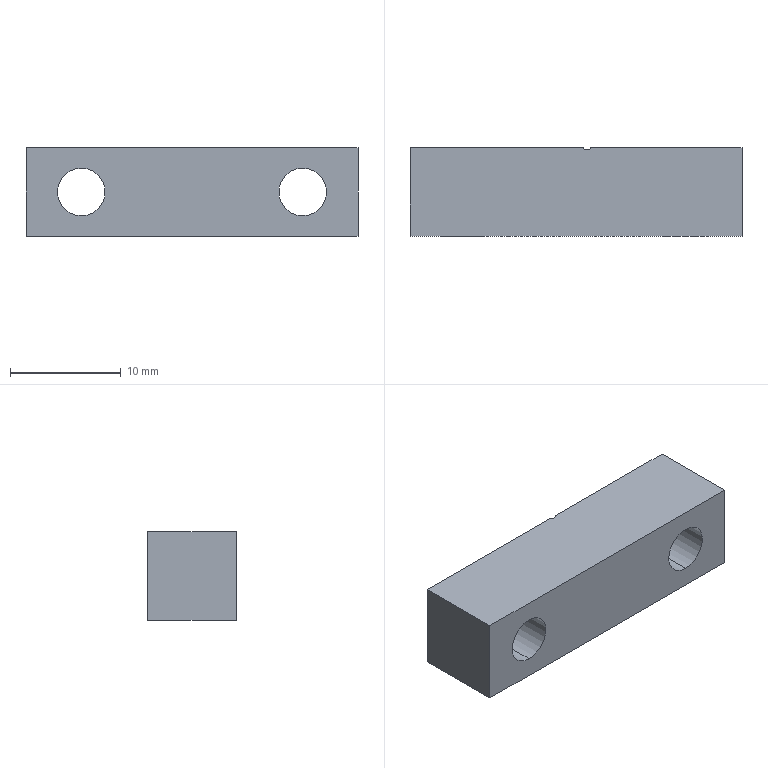Part | SolidWorks | features ICE 2, Extrusion 1 | 1 solid | 12 faces | box 30 x 8 x 8 mm | volume 1687 mm3 | plane 7 | cylinder 5 | commonest cylinder face diameters 4.3 x4 0.8 x1
STEP:
#1=CARTESIAN_POINT('',(-7.907,-5.249,1.85));
#2=VERTEX_POINT('',#1);
#3=CARTESIAN_POINT('',(-7.907,-5.249,6.15));
#4=VERTEX_POINT('',#3);
#5=CARTESIAN_POINT('',(-7.907,-5.249,4.));
#6=DIRECTION('',(0.,1.,0.));
#7=DIRECTION('',(0.,0.,1.));
#8=AXIS2_PLACEMENT_3D('',#5,#6,#7);
#9=CIRCLE('',#8,2.15);
#10=EDGE_CURVE('',#2,#4,#9,.T.);
#11=ORIENTED_EDGE('',*,*,#10,.F.);
#12=CARTESIAN_POINT('',(-7.907,2.751,1.85));
#13=VERTEX_POINT('',#12);
#14=CARTESIAN_POINT('',(-7.907,-5.249,1.85));
#15=DIRECTION('',(0.,1.,0.));
#16=VECTOR('',#15,1000.);
#17=LINE('',#14,#16);
#18=EDGE_CURVE('',#2,#13,#17,.T.);
#19=ORIENTED_EDGE('',*,*,#18,.T.);
#20=CARTESIAN_POINT('',(-7.907,2.751,6.15));
#21=VERTEX_POINT('',#20);
#22=CARTESIAN_POINT('',(-7.907,2.751,4.));
#23=DIRECTION('',(0.,1.,0.));
#24=DIRECTION('',(0.,0.,1.));
#25=AXIS2_PLACEMENT_3D('',#22,#23,#24);
#26=CIRCLE('',#25,2.15);
#27=EDGE_CURVE('',#13,#21,#26,.T.);
#28=ORIENTED_EDGE('',*,*,#27,.T.);
#29=CARTESIAN_POINT('',(-7.907,-5.249,6.15));
#30=DIRECTION('',(0.,1.,0.));
#31=VECTOR('',#30,1000.);
#32=LINE('',#29,#31);
#33=EDGE_CURVE('',#4,#21,#32,.T.);
#34=ORIENTED_EDGE('',*,*,#33,.F.);
#35=EDGE_LOOP('',(#11,#19,#28,#34));
#36=FACE_OUTER_BOUND('',#35,.T.);
#37=CARTESIAN_POINT('',(-7.907,-5.249,4.));
#38=DIRECTION('',(0.,1.,0.));
#39=DIRECTION('',(0.,0.,1.));
#40=AXIS2_PLACEMENT_3D('',#37,#38,#39);
#41=CYLINDRICAL_SURFACE('',#40,2.15);
#42=ADVANCED_FACE('',(#36),#41,.F.);
#43=CARTESIAN_POINT('',(12.093,-5.249,1.85));
#44=VERTEX_POINT('',#43);
#45=CARTESIAN_POINT('',(12.093,-5.249,6.15));
#46=VERTEX_POINT('',#45);
#47=CARTESIAN_POINT('',(12.093,-5.249,4.));
#48=DIRECTION('',(0.,1.,0.));
#49=DIRECTION('',(0.,0.,1.));
#50=AXIS2_PLACEMENT_3D('',#47,#48,#49);
#51=CIRCLE('',#50,2.15);
#52=EDGE_CURVE('',#44,#46,#51,.T.);
#53=ORIENTED_EDGE('',*,*,#52,.F.);
#54=CARTESIAN_POINT('',(12.093,2.751,1.85));
#55=VERTEX_POINT('',#54);
#56=CARTESIAN_POINT('',(12.093,-5.249,1.85));
#57=DIRECTION('',(0.,1.,0.));
#58=VECTOR('',#57,1000.);
#59=LINE('',#56,#58);
#60=EDGE_CURVE('',#44,#55,#59,.T.);
#61=ORIENTED_EDGE('',*,*,#60,.T.);
#62=CARTESIAN_POINT('',(12.093,2.751,6.15));
#63=VERTEX_POINT('',#62);
#64=CARTESIAN_POINT('',(12.093,2.751,4.));
#65=DIRECTION('',(0.,1.,0.));
#66=DIRECTION('',(0.,0.,1.));
#67=AXIS2_PLACEMENT_3D('',#64,#65,#66);
#68=CIRCLE('',#67,2.15);
#69=EDGE_CURVE('',#55,#63,#68,.T.);
#70=ORIENTED_EDGE('',*,*,#69,.T.);
#71=CARTESIAN_POINT('',(12.093,-5.249,6.15));
#72=DIRECTION('',(0.,1.,0.));
#73=VECTOR('',#72,1000.);
#74=LINE('',#71,#73);
#75=EDGE_CURVE('',#46,#63,#74,.T.);
#76=ORIENTED_EDGE('',*,*,#75,.F.);
#77=EDGE_LOOP('',(#53,#61,#70,#76));
#78=FACE_OUTER_BOUND('',#77,.T.);
#79=CARTESIAN_POINT('',(12.093,-5.249,4.));
#80=DIRECTION('',(0.,1.,0.));
#81=DIRECTION('',(0.,0.,1.));
#82=AXIS2_PLACEMENT_3D('',#79,#80,#81);
#83=CYLINDRICAL_SURFACE('',#82,2.15);
#84=ADVANCED_FACE('',(#78),#83,.F.);
#85=CARTESIAN_POINT('',(12.093,2.751,4.));
#86=DIRECTION('',(0.,1.,0.));
#87=DIRECTION('',(0.,0.,1.));
#88=AXIS2_PLACEMENT_3D('',#85,#86,#87);
#89=CIRCLE('',#88,2.15);
#90=EDGE_CURVE('',#63,#55,#89,.T.);
#91=ORIENTED_EDGE('',*,*,#90,.F.);
#92=ORIENTED_EDGE('',*,*,#69,.F.);
#93=EDGE_LOOP('',(#91,#92));
#94=FACE_BOUND('',#93,.T.);
#95=CARTESIAN_POINT('',(17.093,2.751,0.));
#96=VERTEX_POINT('',#95);
#97=CARTESIAN_POINT('',(3.439,2.751,0.));
#98=VERTEX_POINT('',#97);
#99=CARTESIAN_POINT('',(-12.907,2.751,0.));
#100=DIRECTION('',(-1.,0.,0.));
#101=VECTOR('',#100,1000.);
#102=LINE('',#99,#101);
#103=EDGE_CURVE('',#96,#98,#102,.T.);
#104=ORIENTED_EDGE('',*,*,#103,.T.);
#105=CARTESIAN_POINT('',(3.439,2.751,8.));
#106=VERTEX_POINT('',#105);
#107=CARTESIAN_POINT('',(3.439,2.751,0.));
#108=DIRECTION('',(0.,0.,1.));
#109=VECTOR('',#108,1000.);
#110=LINE('',#107,#109);
#111=EDGE_CURVE('',#98,#106,#110,.T.);
#112=ORIENTED_EDGE('',*,*,#111,.T.);
#113=CARTESIAN_POINT('',(17.093,2.751,8.));
#114=VERTEX_POINT('',#113);
#115=CARTESIAN_POINT('',(-12.907,2.751,8.));
#116=DIRECTION('',(-1.,0.,0.));
#117=VECTOR('',#116,1000.);
#118=LINE('',#115,#117);
#119=EDGE_CURVE('',#114,#106,#118,.T.);
#120=ORIENTED_EDGE('',*,*,#119,.F.);
#121=CARTESIAN_POINT('',(17.093,2.751,8.));
#122=DIRECTION('',(0.,0.,-1.));
#123=VECTOR('',#122,1000.);
#124=LINE('',#121,#123);
#125=EDGE_CURVE('',#114,#96,#124,.T.);
#126=ORIENTED_EDGE('',*,*,#125,.T.);
#127=EDGE_LOOP('',(#104,#112,#120,#126));
#128=FACE_OUTER_BOUND('',#127,.T.);
#129=CARTESIAN_POINT('',(-12.907,2.751,8.));
#130=DIRECTION('',(0.,-1.,0.));
#131=DIRECTION('',(0.,0.,-1.));
#132=AXIS2_PLACEMENT_3D('',#129,#130,#131);
#133=PLANE('',#132);
#134=ADVANCED_FACE('',(#94,#128),#133,.F.);
#135=CARTESIAN_POINT('',(-12.907,2.751,0.));
#136=VERTEX_POINT('',#135);
#137=CARTESIAN_POINT('',(-12.907,-5.249,0.));
#138=VERTEX_POINT('',#137);
#139=CARTESIAN_POINT('',(-12.907,2.751,0.));
#140=DIRECTION('',(0.,-1.,0.));
#141=VECTOR('',#140,1000.);
#142=LINE('',#139,#141);
#143=EDGE_CURVE('',#136,#138,#142,.T.);
#144=ORIENTED_EDGE('',*,*,#143,.T.);
#145=CARTESIAN_POINT('',(-12.907,-5.249,8.));
#146=VERTEX_POINT('',#145);
#147=CARTESIAN_POINT('',(-12.907,-5.249,8.));
#148=DIRECTION('',(0.,0.,-1.));
#149=VECTOR('',#148,1000.);
#150=LINE('',#147,#149);
#151=EDGE_CURVE('',#146,#138,#150,.T.);
#152=ORIENTED_EDGE('',*,*,#151,.F.);
#153=CARTESIAN_POINT('',(-12.907,2.751,8.));
#154=VERTEX_POINT('',#153);
#155=CARTESIAN_POINT('',(-12.907,2.751,8.));
#156=DIRECTION('',(0.,-1.,0.));
#157=VECTOR('',#156,1000.);
#158=LINE('',#155,#157);
#159=EDGE_CURVE('',#154,#146,#158,.T.);
#160=ORIENTED_EDGE('',*,*,#159,.F.);
#161=CARTESIAN_POINT('',(-12.907,2.751,8.));
#162=DIRECTION('',(0.,0.,-1.));
#163=VECTOR('',#162,1000.);
#164=LINE('',#161,#163);
#165=EDGE_CURVE('',#154,#136,#164,.T.);
#166=ORIENTED_EDGE('',*,*,#165,.T.);
#167=EDGE_LOOP('',(#144,#152,#160,#166));
#168=FACE_OUTER_BOUND('',#167,.T.);
#169=CARTESIAN_POINT('',(-12.907,2.751,8.));
#170=DIRECTION('',(1.,0.,0.));
#171=DIRECTION('',(0.,0.,-1.));
#172=AXIS2_PLACEMENT_3D('',#169,#170,#171);
#173=PLANE('',#172);
#174=ADVANCED_FACE('',(#168),#173,.F.);
#175=CARTESIAN_POINT('',(-7.907,-5.249,4.));
#176=DIRECTION('',(0.,1.,0.));
#177=DIRECTION('',(0.,0.,1.));
#178=AXIS2_PLACEMENT_3D('',#175,#176,#177);
#179=CIRCLE('',#178,2.15);
#180=EDGE_CURVE('',#4,#2,#179,.T.);
#181=ORIENTED_EDGE('',*,*,#180,.T.);
#182=ORIENTED_EDGE('',*,*,#10,.T.);
#183=EDGE_LOOP('',(#181,#182));
#184=FACE_BOUND('',#183,.T.);
#185=CARTESIAN_POINT('',(12.093,-5.249,4.));
#186=DIRECTION('',(0.,1.,0.));
#187=DIRECTION('',(0.,0.,1.));
#188=AXIS2_PLACEMENT_3D('',#185,#186,#187);
#189=CIRCLE('',#188,2.15);
#190=EDGE_CURVE('',#46,#44,#189,.T.);
#191=ORIENTED_EDGE('',*,*,#190,.T.);
#192=ORIENTED_EDGE('',*,*,#52,.T.);
#193=EDGE_LOOP('',(#191,#192));
#194=FACE_BOUND('',#193,.T.);
#195=CARTESIAN_POINT('',(17.093,-5.249,0.));
#196=VERTEX_POINT('',#195);
#197=CARTESIAN_POINT('',(-12.907,-5.249,0.));
#198=DIRECTION('',(1.,0.,0.));
#199=VECTOR('',#198,1000.);
#200=LINE('',#197,#199);
#201=EDGE_CURVE('',#138,#196,#200,.T.);
#202=ORIENTED_EDGE('',*,*,#201,.T.);
#203=CARTESIAN_POINT('',(17.093,-5.249,8.));
#204=VERTEX_POINT('',#203);
#205=CARTESIAN_POINT('',(17.093,-5.249,8.));
#206=DIRECTION('',(0.,0.,-1.));
#207=VECTOR('',#206,1000.);
#208=LINE('',#205,#207);
#209=EDGE_CURVE('',#204,#196,#208,.T.);
#210=ORIENTED_EDGE('',*,*,#209,.F.);
#211=CARTESIAN_POINT('',(-12.907,-5.249,8.));
#212=DIRECTION('',(1.,0.,0.));
#213=VECTOR('',#212,1000.);
#214=LINE('',#211,#213);
#215=EDGE_CURVE('',#146,#204,#214,.T.);
#216=ORIENTED_EDGE('',*,*,#215,.F.);
#217=ORIENTED_EDGE('',*,*,#151,.T.);
#218=EDGE_LOOP('',(#202,#210,#216,#217));
#219=FACE_OUTER_BOUND('',#218,.T.);
#220=CARTESIAN_POINT('',(-12.907,-5.249,8.));
#221=DIRECTION('',(0.,1.,0.));
#222=DIRECTION('',(0.,0.,1.));
#223=AXIS2_PLACEMENT_3D('',#220,#221,#222);
#224=PLANE('',#223);
#225=ADVANCED_FACE('',(#184,#194,#219),#224,.F.);
#226=CARTESIAN_POINT('',(17.093,2.751,0.));
#227=DIRECTION('',(0.,1.,0.));
#228=VECTOR('',#227,1000.);
#229=LINE('',#226,#228);
#230=EDGE_CURVE('',#196,#96,#229,.T.);
#231=ORIENTED_EDGE('',*,*,#230,.T.);
#232=ORIENTED_EDGE('',*,*,#125,.F.);
#233=CARTESIAN_POINT('',(17.093,2.751,8.));
#234=DIRECTION('',(0.,1.,0.));
#235=VECTOR('',#234,1000.);
#236=LINE('',#233,#235);
#237=EDGE_CURVE('',#204,#114,#236,.T.);
#238=ORIENTED_EDGE('',*,*,#237,.F.);
#239=ORIENTED_EDGE('',*,*,#209,.T.);
#240=EDGE_LOOP('',(#231,#232,#238,#239));
#241=FACE_OUTER_BOUND('',#240,.T.);
#242=CARTESIAN_POINT('',(17.093,2.751,8.));
#243=DIRECTION('',(-1.,0.,0.));
#244=DIRECTION('',(0.,0.,1.));
#245=AXIS2_PLACEMENT_3D('',#242,#243,#244);
#246=PLANE('',#245);
#247=ADVANCED_FACE('',(#241),#246,.F.);
#248=CARTESIAN_POINT('',(-7.907,2.751,4.));
#249=DIRECTION('',(0.,1.,0.));
#250=DIRECTION('',(0.,0.,1.));
#251=AXIS2_PLACEMENT_3D('',#248,#249,#250);
#252=CIRCLE('',#251,2.15);
#253=EDGE_CURVE('',#21,#13,#252,.T.);
#254=ORIENTED_EDGE('',*,*,#253,.F.);
#255=ORIENTED_EDGE('',*,*,#27,.F.);
#256=EDGE_LOOP('',(#254,#255));
#257=FACE_BOUND('',#256,.T.);
#258=CARTESIAN_POINT('',(2.747,2.751,8.));
#259=VERTEX_POINT('',#258);
#260=CARTESIAN_POINT('',(-12.907,2.751,8.));
#261=DIRECTION('',(-1.,0.,0.));
#262=VECTOR('',#261,1000.);
#263=LINE('',#260,#262);
#264=EDGE_CURVE('',#259,#154,#263,.T.);
#265=ORIENTED_EDGE('',*,*,#264,.F.);
#266=CARTESIAN_POINT('',(2.747,2.751,0.));
#267=VERTEX_POINT('',#266);
#268=CARTESIAN_POINT('',(2.747,2.751,0.));
#269=DIRECTION('',(0.,0.,1.));
#270=VECTOR('',#269,1000.);
#271=LINE('',#268,#270);
#272=EDGE_CURVE('',#267,#259,#271,.T.);
#273=ORIENTED_EDGE('',*,*,#272,.F.);
#274=CARTESIAN_POINT('',(-12.907,2.751,0.));
#275=DIRECTION('',(-1.,0.,0.));
#276=VECTOR('',#275,1000.);
#277=LINE('',#274,#276);
#278=EDGE_CURVE('',#267,#136,#277,.T.);
#279=ORIENTED_EDGE('',*,*,#278,.T.);
#280=ORIENTED_EDGE('',*,*,#165,.F.);
#281=EDGE_LOOP('',(#265,#273,#279,#280));
#282=FACE_OUTER_BOUND('',#281,.T.);
#283=CARTESIAN_POINT('',(-12.907,2.751,8.));
#284=DIRECTION('',(0.,-1.,0.));
#285=DIRECTION('',(0.,0.,-1.));
#286=AXIS2_PLACEMENT_3D('',#283,#284,#285);
#287=PLANE('',#286);
#288=ADVANCED_FACE('',(#257,#282),#287,.F.);
#289=CARTESIAN_POINT('',(3.093,2.951,8.));
#290=DIRECTION('',(0.,0.,1.));
#291=DIRECTION('',(1.,0.,0.));
#292=AXIS2_PLACEMENT_3D('',#289,#290,#291);
#293=CIRCLE('',#292,0.4);
#294=EDGE_CURVE('',#259,#106,#293,.T.);
#295=ORIENTED_EDGE('',*,*,#294,.F.);
#296=ORIENTED_EDGE('',*,*,#264,.T.);
#297=ORIENTED_EDGE('',*,*,#159,.T.);
#298=ORIENTED_EDGE('',*,*,#215,.T.);
#299=ORIENTED_EDGE('',*,*,#237,.T.);
#300=ORIENTED_EDGE('',*,*,#119,.T.);
#301=EDGE_LOOP('',(#295,#296,#297,#298,#299,#300));
#302=FACE_OUTER_BOUND('',#301,.T.);
#303=CARTESIAN_POINT('',(0.,0.,8.));
#304=DIRECTION('',(0.,0.,1.));
#305=DIRECTION('',(1.,0.,0.));
#306=AXIS2_PLACEMENT_3D('',#303,#304,#305);
#307=PLANE('',#306);
#308=ADVANCED_FACE('',(#302),#307,.T.);
#309=ORIENTED_EDGE('',*,*,#278,.F.);
#310=CARTESIAN_POINT('',(3.093,2.951,0.));
#311=DIRECTION('',(0.,0.,1.));
#312=DIRECTION('',(1.,0.,0.));
#313=AXIS2_PLACEMENT_3D('',#310,#311,#312);
#314=CIRCLE('',#313,0.4);
#315=EDGE_CURVE('',#267,#98,#314,.T.);
#316=ORIENTED_EDGE('',*,*,#315,.T.);
#317=ORIENTED_EDGE('',*,*,#103,.F.);
#318=ORIENTED_EDGE('',*,*,#230,.F.);
#319=ORIENTED_EDGE('',*,*,#201,.F.);
#320=ORIENTED_EDGE('',*,*,#143,.F.);
#321=EDGE_LOOP('',(#309,#316,#317,#318,#319,#320));
#322=FACE_OUTER_BOUND('',#321,.T.);
#323=CARTESIAN_POINT('',(0.,0.,0.));
#324=DIRECTION('',(0.,0.,1.));
#325=DIRECTION('',(1.,0.,0.));
#326=AXIS2_PLACEMENT_3D('',#323,#324,#325);
#327=PLANE('',#326);
#328=ADVANCED_FACE('',(#322),#327,.F.);
#329=ORIENTED_EDGE('',*,*,#60,.F.);
#330=ORIENTED_EDGE('',*,*,#190,.F.);
#331=ORIENTED_EDGE('',*,*,#75,.T.);
#332=ORIENTED_EDGE('',*,*,#90,.T.);
#333=EDGE_LOOP('',(#329,#330,#331,#332));
#334=FACE_OUTER_BOUND('',#333,.T.);
#335=CARTESIAN_POINT('',(12.093,-5.249,4.));
#336=DIRECTION('',(0.,1.,0.));
#337=DIRECTION('',(0.,0.,1.));
#338=AXIS2_PLACEMENT_3D('',#335,#336,#337);
#339=CYLINDRICAL_SURFACE('',#338,2.15);
#340=ADVANCED_FACE('',(#334),#339,.F.);
#341=ORIENTED_EDGE('',*,*,#18,.F.);
#342=ORIENTED_EDGE('',*,*,#180,.F.);
#343=ORIENTED_EDGE('',*,*,#33,.T.);
#344=ORIENTED_EDGE('',*,*,#253,.T.);
#345=EDGE_LOOP('',(#341,#342,#343,#344));
#346=FACE_OUTER_BOUND('',#345,.T.);
#347=CARTESIAN_POINT('',(-7.907,-5.249,4.));
#348=DIRECTION('',(0.,1.,0.));
#349=DIRECTION('',(0.,0.,1.));
#350=AXIS2_PLACEMENT_3D('',#347,#348,#349);
#351=CYLINDRICAL_SURFACE('',#350,2.15);
#352=ADVANCED_FACE('',(#346),#351,.F.);
#353=ORIENTED_EDGE('',*,*,#294,.T.);
#354=ORIENTED_EDGE('',*,*,#111,.F.);
#355=ORIENTED_EDGE('',*,*,#315,.F.);
#356=ORIENTED_EDGE('',*,*,#272,.T.);
#357=EDGE_LOOP('',(#353,#354,#355,#356));
#358=FACE_OUTER_BOUND('',#357,.T.);
#359=CARTESIAN_POINT('',(3.093,2.951,0.));
#360=DIRECTION('',(0.,0.,1.));
#361=DIRECTION('',(1.,0.,0.));
#362=AXIS2_PLACEMENT_3D('',#359,#360,#361);
#363=CYLINDRICAL_SURFACE('',#362,0.4);
#364=ADVANCED_FACE('',(#358),#363,.F.);
#365=CLOSED_SHELL('',(#42,#84,#134,#174,#225,#247,#288,#308,#328,#340,#352,#364));
#366=MANIFOLD_SOLID_BREP('',#365);
#367=CARTESIAN_POINT('',(0.,0.,0.));
#368=DIRECTION('',(0.,0.,1.));
#369=DIRECTION('',(1.,0.,0.));
#370=AXIS2_PLACEMENT_3D('',#367,#368,#369);
#371=(LENGTH_UNIT()NAMED_UNIT(*)SI_UNIT(.MILLI.,.METRE.));
#372=UNCERTAINTY_MEASURE_WITH_UNIT(LENGTH_MEASURE(0.00001),#371,'','');
#373=(NAMED_UNIT(*)PLANE_ANGLE_UNIT()SI_UNIT($,.RADIAN.));
#374=(NAMED_UNIT(*)SI_UNIT($,.STERADIAN.)SOLID_ANGLE_UNIT());
#375=(GEOMETRIC_REPRESENTATION_CONTEXT(3)GLOBAL_UNCERTAINTY_ASSIGNED_CONTEXT((#372))GLOBAL_UNIT_ASSIGNED_CONTEXT((#371,#373,#374))REPRESENTATION_CONTEXT('',''));
#376=ADVANCED_BREP_SHAPE_REPRESENTATION('',(#366,#370),#375);